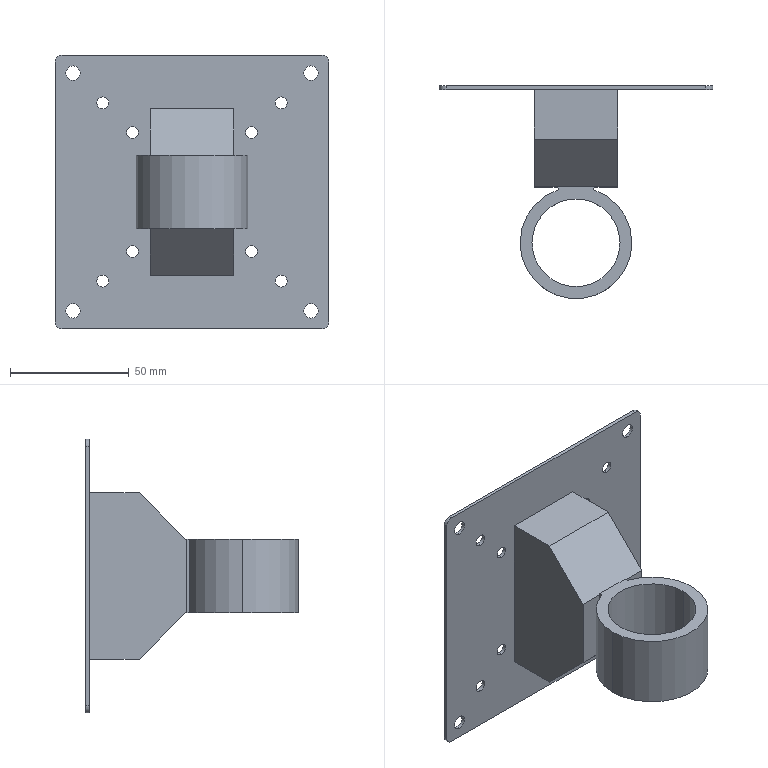Part | SolidWorks | features ICE 5, Chamfer 1, Extrusion 1, Fillet 1 | 1 solid | 53 faces | box 115 x 89.5 x 115 mm | volume 126511 mm3 | cylinder 33 | plane 20 | commonest cylinder face diameters 5 x16 6 x12 47 x3 37 x2